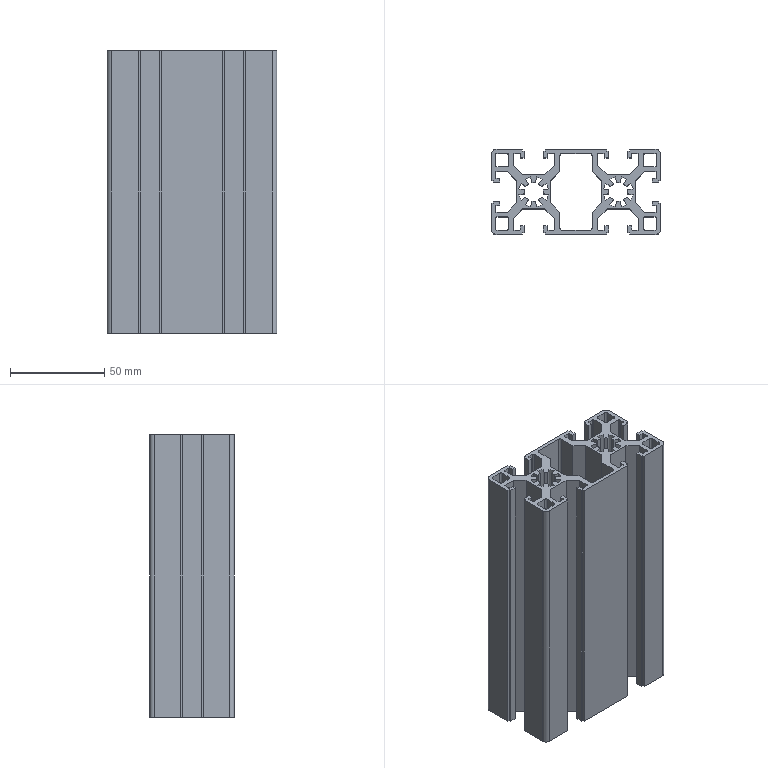Part | STEP file | OB4590-L2 | 1 solid | 256 faces | box 90 x 45 x 150 mm | volume 191709 mm3 | plane 174 | cylinder 82 | commonest cylinder face diameters 1 x24 2 x20 10.2 x18 16 x16 5 x4